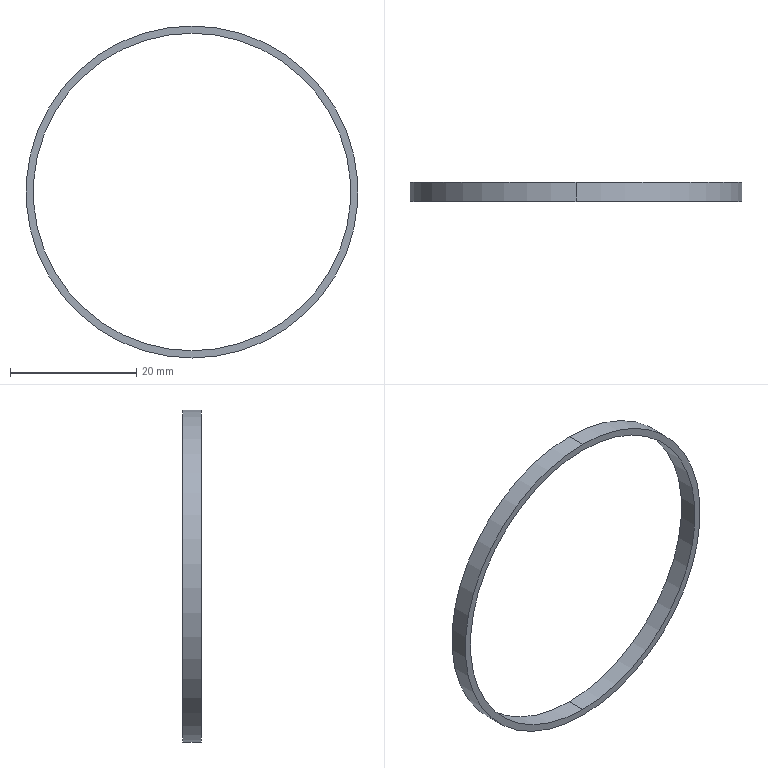Part | SolidWorks | features Extrusion 1 | 1 solid | 6 faces | box 52.5 x 3 x 52.5 mm | volume 556.557 mm3 | cylinder 4 | plane 2 | commonest cylinder face diameters 50.2 x2 52.5 x2
STEP:
#1=CARTESIAN_POINT('',(0.,3.,-25.1));
#2=VERTEX_POINT('',#1);
#3=CARTESIAN_POINT('',(0.,3.,25.1));
#4=VERTEX_POINT('',#3);
#5=CARTESIAN_POINT('',(0.,3.,0.));
#6=DIRECTION('',(0.,1.,0.));
#7=DIRECTION('',(0.,0.,1.));
#8=AXIS2_PLACEMENT_3D('',#5,#6,#7);
#9=CIRCLE('',#8,25.1);
#10=EDGE_CURVE('',#2,#4,#9,.T.);
#11=ORIENTED_EDGE('',*,*,#10,.T.);
#12=CARTESIAN_POINT('',(0.,0.,25.1));
#13=VERTEX_POINT('',#12);
#14=CARTESIAN_POINT('',(0.,3.,25.1));
#15=DIRECTION('',(0.,-1.,0.));
#16=VECTOR('',#15,1000.);
#17=LINE('',#14,#16);
#18=EDGE_CURVE('',#4,#13,#17,.T.);
#19=ORIENTED_EDGE('',*,*,#18,.T.);
#20=CARTESIAN_POINT('',(0.,0.,-25.1));
#21=VERTEX_POINT('',#20);
#22=CARTESIAN_POINT('',(0.,0.,0.));
#23=DIRECTION('',(0.,1.,0.));
#24=DIRECTION('',(0.,0.,1.));
#25=AXIS2_PLACEMENT_3D('',#22,#23,#24);
#26=CIRCLE('',#25,25.1);
#27=EDGE_CURVE('',#21,#13,#26,.T.);
#28=ORIENTED_EDGE('',*,*,#27,.F.);
#29=CARTESIAN_POINT('',(0.,3.,-25.1));
#30=DIRECTION('',(0.,-1.,0.));
#31=VECTOR('',#30,1000.);
#32=LINE('',#29,#31);
#33=EDGE_CURVE('',#2,#21,#32,.T.);
#34=ORIENTED_EDGE('',*,*,#33,.F.);
#35=EDGE_LOOP('',(#11,#19,#28,#34));
#36=FACE_OUTER_BOUND('',#35,.T.);
#37=CARTESIAN_POINT('',(0.,3.,0.));
#38=DIRECTION('',(0.,-1.,0.));
#39=DIRECTION('',(0.,0.,-1.));
#40=AXIS2_PLACEMENT_3D('',#37,#38,#39);
#41=CYLINDRICAL_SURFACE('',#40,25.1);
#42=ADVANCED_FACE('',(#36),#41,.F.);
#43=CARTESIAN_POINT('',(0.,3.,26.25));
#44=VERTEX_POINT('',#43);
#45=CARTESIAN_POINT('',(0.,3.,-26.25));
#46=VERTEX_POINT('',#45);
#47=CARTESIAN_POINT('',(0.,3.,0.));
#48=DIRECTION('',(0.,1.,0.));
#49=DIRECTION('',(0.,0.,1.));
#50=AXIS2_PLACEMENT_3D('',#47,#48,#49);
#51=CIRCLE('',#50,26.25);
#52=EDGE_CURVE('',#44,#46,#51,.T.);
#53=ORIENTED_EDGE('',*,*,#52,.F.);
#54=CARTESIAN_POINT('',(0.,0.,26.25));
#55=VERTEX_POINT('',#54);
#56=CARTESIAN_POINT('',(0.,3.,26.25));
#57=DIRECTION('',(0.,-1.,0.));
#58=VECTOR('',#57,1000.);
#59=LINE('',#56,#58);
#60=EDGE_CURVE('',#44,#55,#59,.T.);
#61=ORIENTED_EDGE('',*,*,#60,.T.);
#62=CARTESIAN_POINT('',(0.,0.,-26.25));
#63=VERTEX_POINT('',#62);
#64=CARTESIAN_POINT('',(0.,0.,0.));
#65=DIRECTION('',(0.,1.,0.));
#66=DIRECTION('',(0.,0.,1.));
#67=AXIS2_PLACEMENT_3D('',#64,#65,#66);
#68=CIRCLE('',#67,26.25);
#69=EDGE_CURVE('',#55,#63,#68,.T.);
#70=ORIENTED_EDGE('',*,*,#69,.T.);
#71=CARTESIAN_POINT('',(0.,3.,-26.25));
#72=DIRECTION('',(0.,-1.,0.));
#73=VECTOR('',#72,1000.);
#74=LINE('',#71,#73);
#75=EDGE_CURVE('',#46,#63,#74,.T.);
#76=ORIENTED_EDGE('',*,*,#75,.F.);
#77=EDGE_LOOP('',(#53,#61,#70,#76));
#78=FACE_OUTER_BOUND('',#77,.T.);
#79=CARTESIAN_POINT('',(0.,3.,0.));
#80=DIRECTION('',(0.,-1.,0.));
#81=DIRECTION('',(0.,0.,-1.));
#82=AXIS2_PLACEMENT_3D('',#79,#80,#81);
#83=CYLINDRICAL_SURFACE('',#82,26.25);
#84=ADVANCED_FACE('',(#78),#83,.T.);
#85=CARTESIAN_POINT('',(0.,3.,0.));
#86=DIRECTION('',(0.,1.,0.));
#87=DIRECTION('',(0.,0.,1.));
#88=AXIS2_PLACEMENT_3D('',#85,#86,#87);
#89=CIRCLE('',#88,26.25);
#90=EDGE_CURVE('',#46,#44,#89,.T.);
#91=ORIENTED_EDGE('',*,*,#90,.T.);
#92=ORIENTED_EDGE('',*,*,#52,.T.);
#93=EDGE_LOOP('',(#91,#92));
#94=FACE_OUTER_BOUND('',#93,.T.);
#95=ORIENTED_EDGE('',*,*,#10,.F.);
#96=CARTESIAN_POINT('',(0.,3.,0.));
#97=DIRECTION('',(0.,1.,0.));
#98=DIRECTION('',(0.,0.,1.));
#99=AXIS2_PLACEMENT_3D('',#96,#97,#98);
#100=CIRCLE('',#99,25.1);
#101=EDGE_CURVE('',#4,#2,#100,.T.);
#102=ORIENTED_EDGE('',*,*,#101,.F.);
#103=EDGE_LOOP('',(#95,#102));
#104=FACE_BOUND('',#103,.T.);
#105=CARTESIAN_POINT('',(0.,3.,0.));
#106=DIRECTION('',(0.,1.,0.));
#107=DIRECTION('',(0.,0.,1.));
#108=AXIS2_PLACEMENT_3D('',#105,#106,#107);
#109=PLANE('',#108);
#110=ADVANCED_FACE('',(#94,#104),#109,.T.);
#111=CARTESIAN_POINT('',(0.,0.,0.));
#112=DIRECTION('',(0.,1.,0.));
#113=DIRECTION('',(0.,0.,1.));
#114=AXIS2_PLACEMENT_3D('',#111,#112,#113);
#115=CIRCLE('',#114,26.25);
#116=EDGE_CURVE('',#63,#55,#115,.T.);
#117=ORIENTED_EDGE('',*,*,#116,.F.);
#118=ORIENTED_EDGE('',*,*,#69,.F.);
#119=EDGE_LOOP('',(#117,#118));
#120=FACE_OUTER_BOUND('',#119,.T.);
#121=ORIENTED_EDGE('',*,*,#27,.T.);
#122=CARTESIAN_POINT('',(0.,0.,0.));
#123=DIRECTION('',(0.,1.,0.));
#124=DIRECTION('',(0.,0.,1.));
#125=AXIS2_PLACEMENT_3D('',#122,#123,#124);
#126=CIRCLE('',#125,25.1);
#127=EDGE_CURVE('',#13,#21,#126,.T.);
#128=ORIENTED_EDGE('',*,*,#127,.T.);
#129=EDGE_LOOP('',(#121,#128));
#130=FACE_BOUND('',#129,.T.);
#131=CARTESIAN_POINT('',(0.,0.,0.));
#132=DIRECTION('',(0.,1.,0.));
#133=DIRECTION('',(0.,0.,1.));
#134=AXIS2_PLACEMENT_3D('',#131,#132,#133);
#135=PLANE('',#134);
#136=ADVANCED_FACE('',(#120,#130),#135,.F.);
#137=ORIENTED_EDGE('',*,*,#60,.F.);
#138=ORIENTED_EDGE('',*,*,#90,.F.);
#139=ORIENTED_EDGE('',*,*,#75,.T.);
#140=ORIENTED_EDGE('',*,*,#116,.T.);
#141=EDGE_LOOP('',(#137,#138,#139,#140));
#142=FACE_OUTER_BOUND('',#141,.T.);
#143=CARTESIAN_POINT('',(0.,3.,0.));
#144=DIRECTION('',(0.,-1.,0.));
#145=DIRECTION('',(0.,0.,-1.));
#146=AXIS2_PLACEMENT_3D('',#143,#144,#145);
#147=CYLINDRICAL_SURFACE('',#146,26.25);
#148=ADVANCED_FACE('',(#142),#147,.T.);
#149=ORIENTED_EDGE('',*,*,#18,.F.);
#150=ORIENTED_EDGE('',*,*,#101,.T.);
#151=ORIENTED_EDGE('',*,*,#33,.T.);
#152=ORIENTED_EDGE('',*,*,#127,.F.);
#153=EDGE_LOOP('',(#149,#150,#151,#152));
#154=FACE_OUTER_BOUND('',#153,.T.);
#155=CARTESIAN_POINT('',(0.,3.,0.));
#156=DIRECTION('',(0.,-1.,0.));
#157=DIRECTION('',(0.,0.,-1.));
#158=AXIS2_PLACEMENT_3D('',#155,#156,#157);
#159=CYLINDRICAL_SURFACE('',#158,25.1);
#160=ADVANCED_FACE('',(#154),#159,.F.);
#161=CLOSED_SHELL('',(#42,#84,#110,#136,#148,#160));
#162=MANIFOLD_SOLID_BREP('',#161);
#163=CARTESIAN_POINT('',(0.,0.,0.));
#164=DIRECTION('',(0.,0.,1.));
#165=DIRECTION('',(1.,0.,0.));
#166=AXIS2_PLACEMENT_3D('',#163,#164,#165);
#167=(LENGTH_UNIT()NAMED_UNIT(*)SI_UNIT(.MILLI.,.METRE.));
#168=UNCERTAINTY_MEASURE_WITH_UNIT(LENGTH_MEASURE(0.00001),#167,'','');
#169=(NAMED_UNIT(*)PLANE_ANGLE_UNIT()SI_UNIT($,.RADIAN.));
#170=(NAMED_UNIT(*)SI_UNIT($,.STERADIAN.)SOLID_ANGLE_UNIT());
#171=(GEOMETRIC_REPRESENTATION_CONTEXT(3)GLOBAL_UNCERTAINTY_ASSIGNED_CONTEXT((#168))GLOBAL_UNIT_ASSIGNED_CONTEXT((#167,#169,#170))REPRESENTATION_CONTEXT('',''));
#172=ADVANCED_BREP_SHAPE_REPRESENTATION('',(#162,#166),#171);